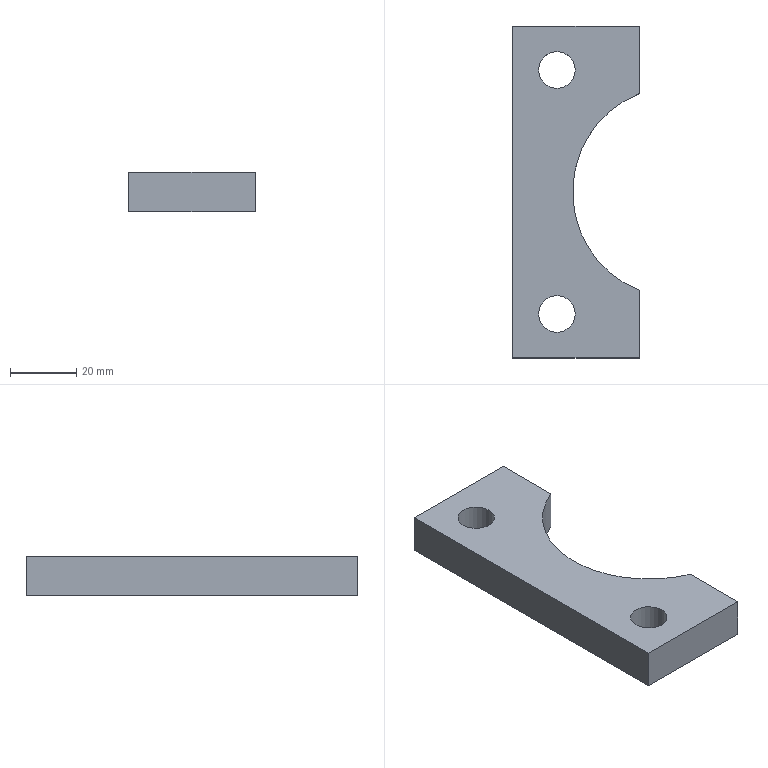Part | NX | features solid 2 | 1 solid | 10 faces | box 38 x 100 x 12 mm | volume 33012 mm3 | plane 7 | cylinder 3 | commonest cylinder face diameters 11 x2 64 x1
STEP:
#1=CARTESIAN_POINT('',(1368.,475.335,385.));
#2=VERTEX_POINT('',#1);
#3=CARTESIAN_POINT('',(1368.,475.335,373.));
#4=VERTEX_POINT('',#3);
#5=CARTESIAN_POINT('',(1368.,475.335,379.));
#6=DIRECTION('',(0.,0.,1.));
#7=VECTOR('',#6,1000.);
#8=LINE('',#5,#7);
#9=EDGE_CURVE('',#2,#4,#8,.F.);
#10=ORIENTED_EDGE('',*,*,#9,.F.);
#11=CARTESIAN_POINT('',(1368.,455.,385.));
#12=VERTEX_POINT('',#11);
#13=CARTESIAN_POINT('',(1368.,555.,385.));
#14=DIRECTION('',(0.,-1.,0.));
#15=VECTOR('',#14,1000.);
#16=LINE('',#13,#15);
#17=EDGE_CURVE('',#2,#12,#16,.T.);
#18=ORIENTED_EDGE('',*,*,#17,.T.);
#19=CARTESIAN_POINT('',(1368.,455.,373.));
#20=VERTEX_POINT('',#19);
#21=CARTESIAN_POINT('',(1368.,455.,373.));
#22=DIRECTION('',(0.,0.,1.));
#23=VECTOR('',#22,1000.);
#24=LINE('',#21,#23);
#25=EDGE_CURVE('',#20,#12,#24,.T.);
#26=ORIENTED_EDGE('',*,*,#25,.F.);
#27=CARTESIAN_POINT('',(1368.,555.,373.));
#28=DIRECTION('',(0.,-1.,0.));
#29=VECTOR('',#28,1000.);
#30=LINE('',#27,#29);
#31=EDGE_CURVE('',#4,#20,#30,.T.);
#32=ORIENTED_EDGE('',*,*,#31,.F.);
#33=EDGE_LOOP('',(#10,#18,#26,#32));
#34=FACE_BOUND('',#33,.T.);
#35=CARTESIAN_POINT('',(1368.,555.,373.));
#36=DIRECTION('',(-1.,0.,0.));
#37=DIRECTION('',(0.,1.,0.));
#38=AXIS2_PLACEMENT_3D('',#35,#36,#37);
#39=PLANE('',#38);
#40=ADVANCED_FACE('',(#34),#39,.F.);
#41=CARTESIAN_POINT('',(1368.,534.665,373.));
#42=VERTEX_POINT('',#41);
#43=CARTESIAN_POINT('',(1368.,534.665,385.));
#44=VERTEX_POINT('',#43);
#45=CARTESIAN_POINT('',(1368.,534.665,379.));
#46=DIRECTION('',(0.,0.,1.));
#47=VECTOR('',#46,1000.);
#48=LINE('',#45,#47);
#49=EDGE_CURVE('',#42,#44,#48,.T.);
#50=ORIENTED_EDGE('',*,*,#49,.F.);
#51=CARTESIAN_POINT('',(1368.,555.,373.));
#52=VERTEX_POINT('',#51);
#53=CARTESIAN_POINT('',(1368.,555.,373.));
#54=DIRECTION('',(0.,-1.,0.));
#55=VECTOR('',#54,1000.);
#56=LINE('',#53,#55);
#57=EDGE_CURVE('',#52,#42,#56,.T.);
#58=ORIENTED_EDGE('',*,*,#57,.F.);
#59=CARTESIAN_POINT('',(1368.,555.,385.));
#60=VERTEX_POINT('',#59);
#61=CARTESIAN_POINT('',(1368.,555.,373.));
#62=DIRECTION('',(0.,0.,1.));
#63=VECTOR('',#62,1000.);
#64=LINE('',#61,#63);
#65=EDGE_CURVE('',#52,#60,#64,.T.);
#66=ORIENTED_EDGE('',*,*,#65,.T.);
#67=CARTESIAN_POINT('',(1368.,555.,385.));
#68=DIRECTION('',(0.,-1.,0.));
#69=VECTOR('',#68,1000.);
#70=LINE('',#67,#69);
#71=EDGE_CURVE('',#60,#44,#70,.T.);
#72=ORIENTED_EDGE('',*,*,#71,.T.);
#73=EDGE_LOOP('',(#50,#58,#66,#72));
#74=FACE_BOUND('',#73,.T.);
#75=CARTESIAN_POINT('',(1368.,555.,373.));
#76=DIRECTION('',(-1.,0.,0.));
#77=DIRECTION('',(0.,1.,0.));
#78=AXIS2_PLACEMENT_3D('',#75,#76,#77);
#79=PLANE('',#78);
#80=ADVANCED_FACE('',(#74),#79,.F.);
#81=CARTESIAN_POINT('',(1348.75,541.75,373.));
#82=VERTEX_POINT('',#81);
#83=CARTESIAN_POINT('',(1343.25,541.75,373.));
#84=DIRECTION('',(0.,0.,1.));
#85=DIRECTION('',(1.,0.,0.));
#86=AXIS2_PLACEMENT_3D('',#83,#84,#85);
#87=CIRCLE('',#86,5.5);
#88=EDGE_CURVE('',#82,#82,#87,.T.);
#89=ORIENTED_EDGE('',*,*,#88,.T.);
#90=EDGE_LOOP('',(#89));
#91=FACE_BOUND('',#90,.T.);
#92=CARTESIAN_POINT('',(1348.75,468.25,373.));
#93=VERTEX_POINT('',#92);
#94=CARTESIAN_POINT('',(1343.25,468.25,373.));
#95=DIRECTION('',(0.,0.,-1.));
#96=DIRECTION('',(1.,0.,0.));
#97=AXIS2_PLACEMENT_3D('',#94,#95,#96);
#98=CIRCLE('',#97,5.5);
#99=EDGE_CURVE('',#93,#93,#98,.T.);
#100=ORIENTED_EDGE('',*,*,#99,.F.);
#101=EDGE_LOOP('',(#100));
#102=FACE_BOUND('',#101,.T.);
#103=CARTESIAN_POINT('',(1380.,505.,373.));
#104=DIRECTION('',(0.,0.,1.));
#105=DIRECTION('',(1.,0.,0.));
#106=AXIS2_PLACEMENT_3D('',#103,#104,#105);
#107=CIRCLE('',#106,32.);
#108=EDGE_CURVE('',#4,#42,#107,.F.);
#109=ORIENTED_EDGE('',*,*,#108,.F.);
#110=ORIENTED_EDGE('',*,*,#31,.T.);
#111=CARTESIAN_POINT('',(1330.,455.,373.));
#112=VERTEX_POINT('',#111);
#113=CARTESIAN_POINT('',(1368.,455.,373.));
#114=DIRECTION('',(-1.,0.,0.));
#115=VECTOR('',#114,1000.);
#116=LINE('',#113,#115);
#117=EDGE_CURVE('',#20,#112,#116,.T.);
#118=ORIENTED_EDGE('',*,*,#117,.T.);
#119=CARTESIAN_POINT('',(1330.,555.,373.));
#120=VERTEX_POINT('',#119);
#121=CARTESIAN_POINT('',(1330.,455.,373.));
#122=DIRECTION('',(0.,1.,0.));
#123=VECTOR('',#122,1000.);
#124=LINE('',#121,#123);
#125=EDGE_CURVE('',#112,#120,#124,.T.);
#126=ORIENTED_EDGE('',*,*,#125,.T.);
#127=CARTESIAN_POINT('',(1330.,555.,373.));
#128=DIRECTION('',(1.,0.,0.));
#129=VECTOR('',#128,1000.);
#130=LINE('',#127,#129);
#131=EDGE_CURVE('',#120,#52,#130,.T.);
#132=ORIENTED_EDGE('',*,*,#131,.T.);
#133=ORIENTED_EDGE('',*,*,#57,.T.);
#134=EDGE_LOOP('',(#109,#110,#118,#126,#132,#133));
#135=FACE_BOUND('',#134,.T.);
#136=CARTESIAN_POINT('',(1330.,555.,373.));
#137=DIRECTION('',(0.,0.,1.));
#138=DIRECTION('',(1.,0.,0.));
#139=AXIS2_PLACEMENT_3D('',#136,#137,#138);
#140=PLANE('',#139);
#141=ADVANCED_FACE('',(#91,#102,#135),#140,.F.);
#142=CARTESIAN_POINT('',(1348.75,541.75,385.));
#143=VERTEX_POINT('',#142);
#144=CARTESIAN_POINT('',(1343.25,541.75,385.));
#145=DIRECTION('',(0.,0.,1.));
#146=DIRECTION('',(1.,0.,0.));
#147=AXIS2_PLACEMENT_3D('',#144,#145,#146);
#148=CIRCLE('',#147,5.5);
#149=EDGE_CURVE('',#143,#143,#148,.T.);
#150=ORIENTED_EDGE('',*,*,#149,.F.);
#151=EDGE_LOOP('',(#150));
#152=FACE_BOUND('',#151,.T.);
#153=CARTESIAN_POINT('',(1348.75,468.25,385.));
#154=VERTEX_POINT('',#153);
#155=CARTESIAN_POINT('',(1343.25,468.25,385.));
#156=DIRECTION('',(0.,0.,-1.));
#157=DIRECTION('',(1.,0.,0.));
#158=AXIS2_PLACEMENT_3D('',#155,#156,#157);
#159=CIRCLE('',#158,5.5);
#160=EDGE_CURVE('',#154,#154,#159,.T.);
#161=ORIENTED_EDGE('',*,*,#160,.T.);
#162=EDGE_LOOP('',(#161));
#163=FACE_BOUND('',#162,.T.);
#164=ORIENTED_EDGE('',*,*,#17,.F.);
#165=CARTESIAN_POINT('',(1380.,505.,385.));
#166=DIRECTION('',(0.,0.,1.));
#167=DIRECTION('',(1.,0.,0.));
#168=AXIS2_PLACEMENT_3D('',#165,#166,#167);
#169=CIRCLE('',#168,32.);
#170=EDGE_CURVE('',#2,#44,#169,.F.);
#171=ORIENTED_EDGE('',*,*,#170,.T.);
#172=ORIENTED_EDGE('',*,*,#71,.F.);
#173=CARTESIAN_POINT('',(1330.,555.,385.));
#174=VERTEX_POINT('',#173);
#175=CARTESIAN_POINT('',(1330.,555.,385.));
#176=DIRECTION('',(1.,0.,0.));
#177=VECTOR('',#176,1000.);
#178=LINE('',#175,#177);
#179=EDGE_CURVE('',#174,#60,#178,.T.);
#180=ORIENTED_EDGE('',*,*,#179,.F.);
#181=CARTESIAN_POINT('',(1330.,455.,385.));
#182=VERTEX_POINT('',#181);
#183=CARTESIAN_POINT('',(1330.,455.,385.));
#184=DIRECTION('',(0.,1.,0.));
#185=VECTOR('',#184,1000.);
#186=LINE('',#183,#185);
#187=EDGE_CURVE('',#182,#174,#186,.T.);
#188=ORIENTED_EDGE('',*,*,#187,.F.);
#189=CARTESIAN_POINT('',(1368.,455.,385.));
#190=DIRECTION('',(-1.,0.,0.));
#191=VECTOR('',#190,1000.);
#192=LINE('',#189,#191);
#193=EDGE_CURVE('',#12,#182,#192,.T.);
#194=ORIENTED_EDGE('',*,*,#193,.F.);
#195=EDGE_LOOP('',(#164,#171,#172,#180,#188,#194));
#196=FACE_BOUND('',#195,.T.);
#197=CARTESIAN_POINT('',(1330.,555.,385.));
#198=DIRECTION('',(0.,0.,1.));
#199=DIRECTION('',(1.,0.,0.));
#200=AXIS2_PLACEMENT_3D('',#197,#198,#199);
#201=PLANE('',#200);
#202=ADVANCED_FACE('',(#152,#163,#196),#201,.T.);
#203=ORIENTED_EDGE('',*,*,#179,.T.);
#204=ORIENTED_EDGE('',*,*,#65,.F.);
#205=ORIENTED_EDGE('',*,*,#131,.F.);
#206=CARTESIAN_POINT('',(1330.,555.,373.));
#207=DIRECTION('',(0.,0.,1.));
#208=VECTOR('',#207,1000.);
#209=LINE('',#206,#208);
#210=EDGE_CURVE('',#120,#174,#209,.T.);
#211=ORIENTED_EDGE('',*,*,#210,.T.);
#212=EDGE_LOOP('',(#203,#204,#205,#211));
#213=FACE_BOUND('',#212,.T.);
#214=CARTESIAN_POINT('',(1330.,555.,373.));
#215=DIRECTION('',(0.,-1.,0.));
#216=DIRECTION('',(0.,0.,1.));
#217=AXIS2_PLACEMENT_3D('',#214,#215,#216);
#218=PLANE('',#217);
#219=ADVANCED_FACE('',(#213),#218,.F.);
#220=ORIENTED_EDGE('',*,*,#193,.T.);
#221=CARTESIAN_POINT('',(1330.,455.,373.));
#222=DIRECTION('',(0.,0.,1.));
#223=VECTOR('',#222,1000.);
#224=LINE('',#221,#223);
#225=EDGE_CURVE('',#112,#182,#224,.T.);
#226=ORIENTED_EDGE('',*,*,#225,.F.);
#227=ORIENTED_EDGE('',*,*,#117,.F.);
#228=ORIENTED_EDGE('',*,*,#25,.T.);
#229=EDGE_LOOP('',(#220,#226,#227,#228));
#230=FACE_BOUND('',#229,.T.);
#231=CARTESIAN_POINT('',(1368.,455.,373.));
#232=DIRECTION('',(0.,1.,0.));
#233=DIRECTION('',(1.,0.,0.));
#234=AXIS2_PLACEMENT_3D('',#231,#232,#233);
#235=PLANE('',#234);
#236=ADVANCED_FACE('',(#230),#235,.F.);
#237=ORIENTED_EDGE('',*,*,#187,.T.);
#238=ORIENTED_EDGE('',*,*,#210,.F.);
#239=ORIENTED_EDGE('',*,*,#125,.F.);
#240=ORIENTED_EDGE('',*,*,#225,.T.);
#241=EDGE_LOOP('',(#237,#238,#239,#240));
#242=FACE_BOUND('',#241,.T.);
#243=CARTESIAN_POINT('',(1330.,455.,373.));
#244=DIRECTION('',(1.,0.,0.));
#245=DIRECTION('',(0.,-1.,0.));
#246=AXIS2_PLACEMENT_3D('',#243,#244,#245);
#247=PLANE('',#246);
#248=ADVANCED_FACE('',(#242),#247,.F.);
#249=ORIENTED_EDGE('',*,*,#99,.T.);
#250=EDGE_LOOP('',(#249));
#251=FACE_BOUND('',#250,.T.);
#252=ORIENTED_EDGE('',*,*,#160,.F.);
#253=EDGE_LOOP('',(#252));
#254=FACE_BOUND('',#253,.T.);
#255=CARTESIAN_POINT('',(1343.25,468.25,373.));
#256=DIRECTION('',(0.,0.,1.));
#257=DIRECTION('',(1.,0.,0.));
#258=AXIS2_PLACEMENT_3D('',#255,#256,#257);
#259=CYLINDRICAL_SURFACE('',#258,5.5);
#260=ADVANCED_FACE('',(#251,#254),#259,.F.);
#261=ORIENTED_EDGE('',*,*,#88,.F.);
#262=EDGE_LOOP('',(#261));
#263=FACE_BOUND('',#262,.T.);
#264=ORIENTED_EDGE('',*,*,#149,.T.);
#265=EDGE_LOOP('',(#264));
#266=FACE_BOUND('',#265,.T.);
#267=CARTESIAN_POINT('',(1343.25,541.75,373.));
#268=DIRECTION('',(0.,0.,1.));
#269=DIRECTION('',(1.,0.,0.));
#270=AXIS2_PLACEMENT_3D('',#267,#268,#269);
#271=CYLINDRICAL_SURFACE('',#270,5.5);
#272=ADVANCED_FACE('',(#263,#266),#271,.F.);
#273=ORIENTED_EDGE('',*,*,#9,.T.);
#274=ORIENTED_EDGE('',*,*,#108,.T.);
#275=ORIENTED_EDGE('',*,*,#49,.T.);
#276=ORIENTED_EDGE('',*,*,#170,.F.);
#277=EDGE_LOOP('',(#273,#274,#275,#276));
#278=FACE_BOUND('',#277,.T.);
#279=CARTESIAN_POINT('',(1380.,505.,373.));
#280=DIRECTION('',(0.,0.,1.));
#281=DIRECTION('',(1.,0.,0.));
#282=AXIS2_PLACEMENT_3D('',#279,#280,#281);
#283=CYLINDRICAL_SURFACE('',#282,32.);
#284=ADVANCED_FACE('',(#278),#283,.F.);
#285=CLOSED_SHELL('',(#40,#80,#141,#202,#219,#236,#248,#260,#272,#284));
#286=MANIFOLD_SOLID_BREP('',#285);
#287=(LENGTH_UNIT()NAMED_UNIT(*)SI_UNIT(.MILLI.,.METRE.));
#288=UNCERTAINTY_MEASURE_WITH_UNIT(LENGTH_MEASURE(0.00001),#287,'','');
#289=(NAMED_UNIT(*)PLANE_ANGLE_UNIT()SI_UNIT($,.RADIAN.));
#290=(NAMED_UNIT(*)SI_UNIT($,.STERADIAN.)SOLID_ANGLE_UNIT());
#291=(GEOMETRIC_REPRESENTATION_CONTEXT(3)GLOBAL_UNCERTAINTY_ASSIGNED_CONTEXT((#288))GLOBAL_UNIT_ASSIGNED_CONTEXT((#287,#289,#290))REPRESENTATION_CONTEXT('',''));
#292=ADVANCED_BREP_SHAPE_REPRESENTATION('',(#286),#291);